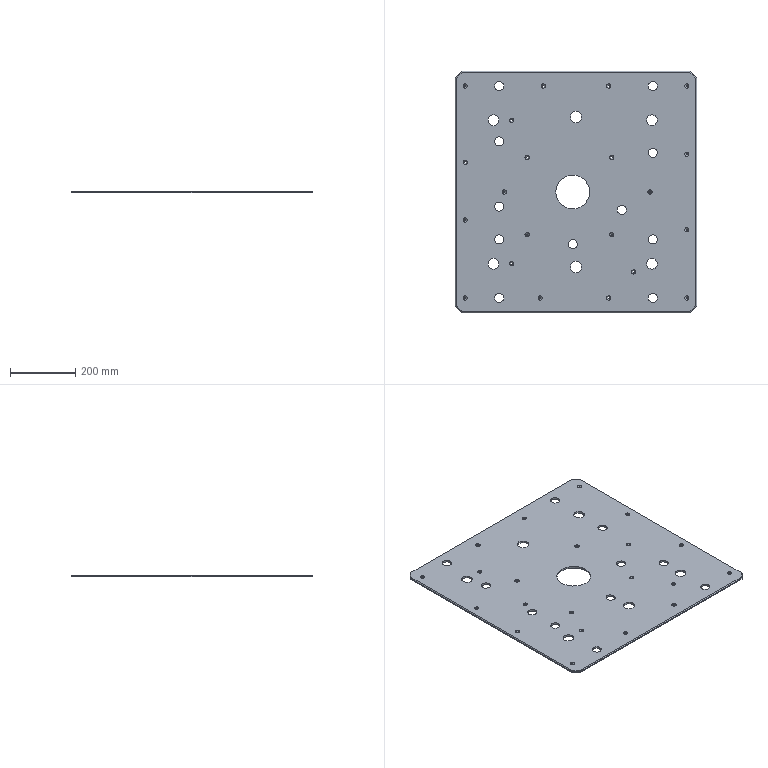Part | Creo | 1 solid | 180 faces | box 740 x 740 x 6 mm | volume 3133769 mm3 | cylinder 120 | cone 42 | plane 18 | commonest cylinder face diameters 6.6 x42 13 x42 28 x22 33 x8 35 x4 104 x2